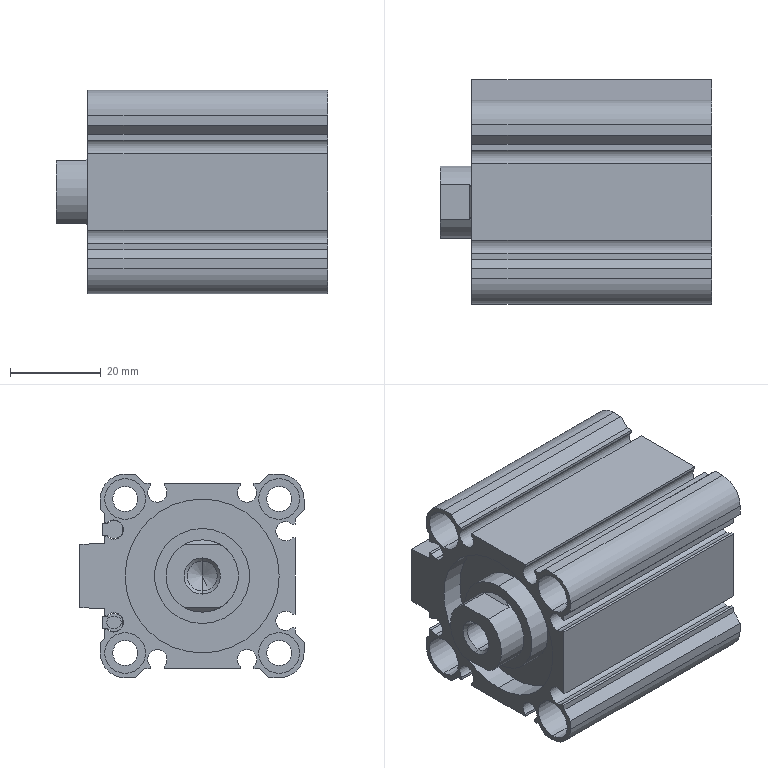Part | SolidWorks | 4 solids | 210 faces | box 60 x 49.5 x 45 mm | volume 70558 mm3 | plane 110 | cylinder 92 | cone 8 | commonest cylinder face diameters 4.26 x18 9 x16 0.6 x8 5.5 x8 4 x6 2 x4